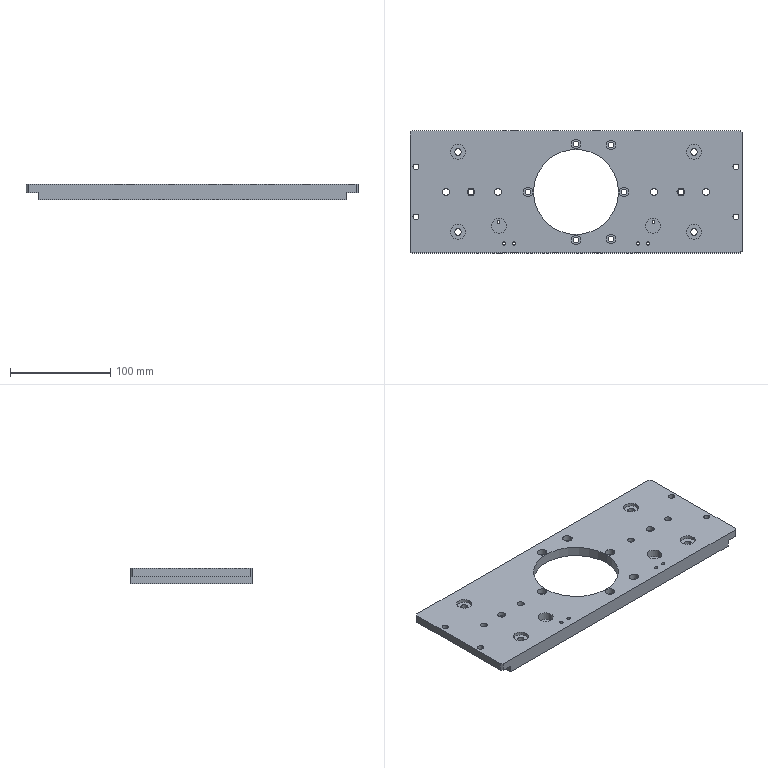Part | STEP file | 227H056237 Under Base | 1 solid | 241 faces | box 332 x 122 x 15 mm | volume 468693 mm3 | cylinder 152 | cone 52 | plane 37 | commonest cylinder face diameters 2.5 x40 2 x16 5.5 x16 9.5 x16 15 x12 3.3 x8